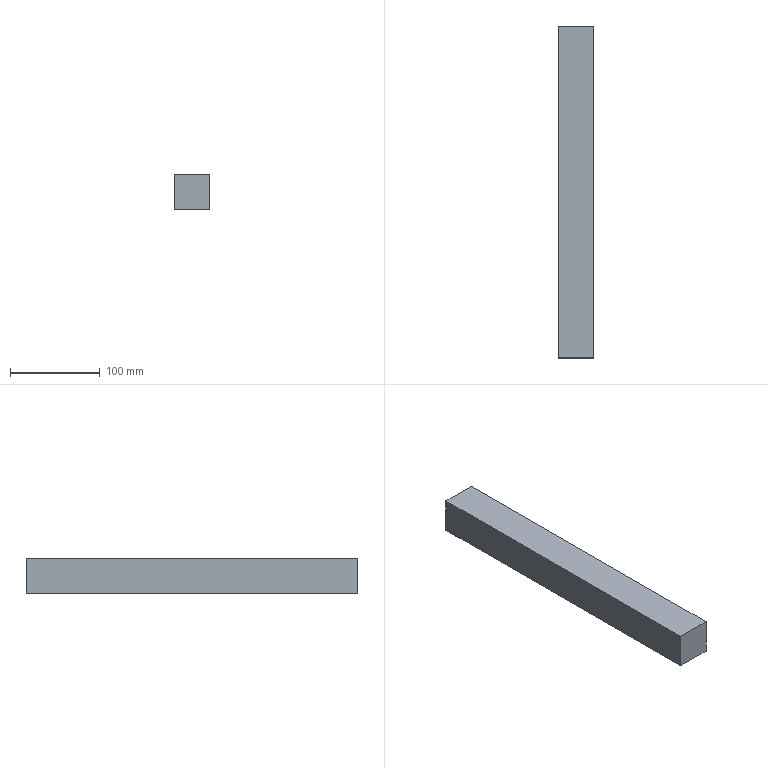Part | NX | 1 solid | 6 faces | box 40 x 370 x 40 mm | volume 592000 mm3 | plane 6
STEP:
#1=CARTESIAN_POINT('',(50.274,48.985,0.));
#2=VERTEX_POINT('',#1);
#3=CARTESIAN_POINT('',(50.274,48.985,-40.));
#4=VERTEX_POINT('',#3);
#5=CARTESIAN_POINT('',(50.274,48.985,0.));
#6=DIRECTION('',(0.,0.,-1.));
#7=VECTOR('',#6,1000.);
#8=LINE('',#5,#7);
#9=EDGE_CURVE('',#2,#4,#8,.T.);
#10=ORIENTED_EDGE('',*,*,#9,.T.);
#11=CARTESIAN_POINT('',(50.274,-321.015,-40.));
#12=VERTEX_POINT('',#11);
#13=CARTESIAN_POINT('',(50.274,48.985,-40.));
#14=DIRECTION('',(0.,-1.,0.));
#15=VECTOR('',#14,1000.);
#16=LINE('',#13,#15);
#17=EDGE_CURVE('',#4,#12,#16,.T.);
#18=ORIENTED_EDGE('',*,*,#17,.T.);
#19=CARTESIAN_POINT('',(50.274,-321.015,0.));
#20=VERTEX_POINT('',#19);
#21=CARTESIAN_POINT('',(50.274,-321.015,0.));
#22=DIRECTION('',(0.,0.,-1.));
#23=VECTOR('',#22,1000.);
#24=LINE('',#21,#23);
#25=EDGE_CURVE('',#20,#12,#24,.T.);
#26=ORIENTED_EDGE('',*,*,#25,.F.);
#27=CARTESIAN_POINT('',(50.274,48.985,0.));
#28=DIRECTION('',(0.,-1.,0.));
#29=VECTOR('',#28,1000.);
#30=LINE('',#27,#29);
#31=EDGE_CURVE('',#2,#20,#30,.T.);
#32=ORIENTED_EDGE('',*,*,#31,.F.);
#33=EDGE_LOOP('',(#10,#18,#26,#32));
#34=FACE_BOUND('',#33,.T.);
#35=CARTESIAN_POINT('',(50.274,48.985,-40.));
#36=DIRECTION('',(-1.,0.,0.));
#37=DIRECTION('',(0.,0.,1.));
#38=AXIS2_PLACEMENT_3D('',#35,#36,#37);
#39=PLANE('',#38);
#40=ADVANCED_FACE('',(#34),#39,.T.);
#41=CARTESIAN_POINT('',(90.274,48.985,-40.));
#42=VERTEX_POINT('',#41);
#43=CARTESIAN_POINT('',(50.274,48.985,-40.));
#44=DIRECTION('',(1.,0.,0.));
#45=VECTOR('',#44,1000.);
#46=LINE('',#43,#45);
#47=EDGE_CURVE('',#4,#42,#46,.T.);
#48=ORIENTED_EDGE('',*,*,#47,.T.);
#49=CARTESIAN_POINT('',(90.274,-321.015,-40.));
#50=VERTEX_POINT('',#49);
#51=CARTESIAN_POINT('',(90.274,48.985,-40.));
#52=DIRECTION('',(0.,-1.,0.));
#53=VECTOR('',#52,1000.);
#54=LINE('',#51,#53);
#55=EDGE_CURVE('',#42,#50,#54,.T.);
#56=ORIENTED_EDGE('',*,*,#55,.T.);
#57=CARTESIAN_POINT('',(50.274,-321.015,-40.));
#58=DIRECTION('',(1.,0.,0.));
#59=VECTOR('',#58,1000.);
#60=LINE('',#57,#59);
#61=EDGE_CURVE('',#12,#50,#60,.T.);
#62=ORIENTED_EDGE('',*,*,#61,.F.);
#63=ORIENTED_EDGE('',*,*,#17,.F.);
#64=EDGE_LOOP('',(#48,#56,#62,#63));
#65=FACE_BOUND('',#64,.T.);
#66=CARTESIAN_POINT('',(90.274,48.985,-40.));
#67=DIRECTION('',(0.,0.,-1.));
#68=DIRECTION('',(0.,-1.,0.));
#69=AXIS2_PLACEMENT_3D('',#66,#67,#68);
#70=PLANE('',#69);
#71=ADVANCED_FACE('',(#65),#70,.T.);
#72=CARTESIAN_POINT('',(90.274,48.985,0.));
#73=VERTEX_POINT('',#72);
#74=CARTESIAN_POINT('',(90.274,48.985,0.));
#75=DIRECTION('',(0.,0.,-1.));
#76=VECTOR('',#75,1000.);
#77=LINE('',#74,#76);
#78=EDGE_CURVE('',#73,#42,#77,.T.);
#79=ORIENTED_EDGE('',*,*,#78,.F.);
#80=CARTESIAN_POINT('',(90.274,-321.015,0.));
#81=VERTEX_POINT('',#80);
#82=CARTESIAN_POINT('',(90.274,48.985,0.));
#83=DIRECTION('',(0.,-1.,0.));
#84=VECTOR('',#83,1000.);
#85=LINE('',#82,#84);
#86=EDGE_CURVE('',#73,#81,#85,.T.);
#87=ORIENTED_EDGE('',*,*,#86,.T.);
#88=CARTESIAN_POINT('',(90.274,-321.015,0.));
#89=DIRECTION('',(0.,0.,-1.));
#90=VECTOR('',#89,1000.);
#91=LINE('',#88,#90);
#92=EDGE_CURVE('',#81,#50,#91,.T.);
#93=ORIENTED_EDGE('',*,*,#92,.T.);
#94=ORIENTED_EDGE('',*,*,#55,.F.);
#95=EDGE_LOOP('',(#79,#87,#93,#94));
#96=FACE_BOUND('',#95,.T.);
#97=CARTESIAN_POINT('',(90.274,48.985,0.));
#98=DIRECTION('',(1.,0.,0.));
#99=DIRECTION('',(0.,1.,0.));
#100=AXIS2_PLACEMENT_3D('',#97,#98,#99);
#101=PLANE('',#100);
#102=ADVANCED_FACE('',(#96),#101,.T.);
#103=CARTESIAN_POINT('',(50.274,48.985,0.));
#104=DIRECTION('',(1.,0.,0.));
#105=VECTOR('',#104,1000.);
#106=LINE('',#103,#105);
#107=EDGE_CURVE('',#2,#73,#106,.T.);
#108=ORIENTED_EDGE('',*,*,#107,.F.);
#109=ORIENTED_EDGE('',*,*,#31,.T.);
#110=CARTESIAN_POINT('',(50.274,-321.015,0.));
#111=DIRECTION('',(1.,0.,0.));
#112=VECTOR('',#111,1000.);
#113=LINE('',#110,#112);
#114=EDGE_CURVE('',#20,#81,#113,.T.);
#115=ORIENTED_EDGE('',*,*,#114,.T.);
#116=ORIENTED_EDGE('',*,*,#86,.F.);
#117=EDGE_LOOP('',(#108,#109,#115,#116));
#118=FACE_BOUND('',#117,.T.);
#119=CARTESIAN_POINT('',(50.274,48.985,0.));
#120=DIRECTION('',(0.,0.,1.));
#121=DIRECTION('',(1.,0.,0.));
#122=AXIS2_PLACEMENT_3D('',#119,#120,#121);
#123=PLANE('',#122);
#124=ADVANCED_FACE('',(#118),#123,.T.);
#125=ORIENTED_EDGE('',*,*,#25,.T.);
#126=ORIENTED_EDGE('',*,*,#61,.T.);
#127=ORIENTED_EDGE('',*,*,#92,.F.);
#128=ORIENTED_EDGE('',*,*,#114,.F.);
#129=EDGE_LOOP('',(#125,#126,#127,#128));
#130=FACE_BOUND('',#129,.T.);
#131=CARTESIAN_POINT('',(78.765,-321.015,-292.061));
#132=DIRECTION('',(0.,-1.,0.));
#133=DIRECTION('',(0.,0.,-1.));
#134=AXIS2_PLACEMENT_3D('',#131,#132,#133);
#135=PLANE('',#134);
#136=ADVANCED_FACE('',(#130),#135,.T.);
#137=ORIENTED_EDGE('',*,*,#107,.T.);
#138=ORIENTED_EDGE('',*,*,#78,.T.);
#139=ORIENTED_EDGE('',*,*,#47,.F.);
#140=ORIENTED_EDGE('',*,*,#9,.F.);
#141=EDGE_LOOP('',(#137,#138,#139,#140));
#142=FACE_BOUND('',#141,.T.);
#143=CARTESIAN_POINT('',(78.765,48.985,-292.061));
#144=DIRECTION('',(0.,-1.,0.));
#145=DIRECTION('',(0.,0.,-1.));
#146=AXIS2_PLACEMENT_3D('',#143,#144,#145);
#147=PLANE('',#146);
#148=ADVANCED_FACE('',(#142),#147,.F.);
#149=CLOSED_SHELL('',(#40,#71,#102,#124,#136,#148));
#150=MANIFOLD_SOLID_BREP('',#149);
#151=(LENGTH_UNIT()NAMED_UNIT(*)SI_UNIT(.MILLI.,.METRE.));
#152=UNCERTAINTY_MEASURE_WITH_UNIT(LENGTH_MEASURE(0.00001),#151,'','');
#153=(NAMED_UNIT(*)PLANE_ANGLE_UNIT()SI_UNIT($,.RADIAN.));
#154=(NAMED_UNIT(*)SI_UNIT($,.STERADIAN.)SOLID_ANGLE_UNIT());
#155=(GEOMETRIC_REPRESENTATION_CONTEXT(3)GLOBAL_UNCERTAINTY_ASSIGNED_CONTEXT((#152))GLOBAL_UNIT_ASSIGNED_CONTEXT((#151,#153,#154))REPRESENTATION_CONTEXT('',''));
#156=ADVANCED_BREP_SHAPE_REPRESENTATION('',(#150),#155);